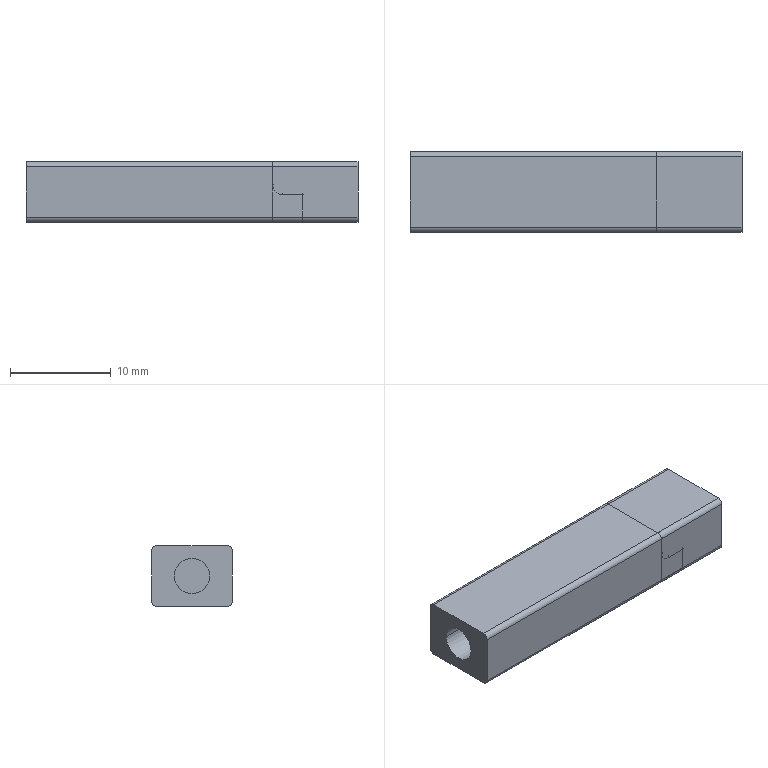NC program | NX | posted with a generic post | part box 33 x 8 x 6 mm
Lines 1895 to 2793 of 11867:
(ZLEVEL_PROFILE_COPY , TOOL : R0.5)
N3746 T13 M6
N3748 G54
N3750 G17 G0 G90 X2.23 Y-1.536 B0. C0. S9500 M3
N3752 G43 Z30. H13
N3754 Z1.5
N3756 G94 G1 X2.302 Y-1.466 Z1.495 F1000.
N3758 X2.547 Y-1.378 Z1.481
N3760 X2.807 Y-1.396 Z1.467
N3762 X3.007 Y-1.494 Z1.456
N3764 X3.168 Y-1.668 Z1.443
N3766 X3.252 Y-1.888 Z1.431
N3768 Y-2.55 Z1.396
N3770 X3.184 Y-2.619 Z1.391
N3772 X2.084 Z1.334
N3774 X2.015 Y-2.55 Z1.328
N3776 Y-1.888 Z1.294
N3778 X2.114 Y-1.647 Z1.28
N3780 X2.302 Y-1.466 Z1.267
N3782 X2.547 Y-1.378 Z1.253
N3784 X2.807 Y-1.396 Z1.239
N3786 X3.007 Y-1.494 Z1.227
N3788 X3.168 Y-1.668 Z1.215
N3790 X3.252 Y-1.888 Z1.203
N3792 Y-2.55 Z1.168
N3794 X3.184 Y-2.619 Z1.163
N3796 X2.084 Z1.105
N3798 X2.015 Y-2.55 Z1.1
N3800 Y-1.888 Z1.066
N3802 X2.114 Y-1.647 Z1.052
N3804 X2.302 Y-1.466 Z1.038
N3806 X2.547 Y-1.378 Z1.025
N3808 X2.807 Y-1.396 Z1.011
N3810 X3.007 Y-1.494 Z0.999
N3812 X3.168 Y-1.668 Z0.987
N3814 X3.252 Y-1.888 Z0.974
N3816 Y-2.55 Z0.94
N3818 X3.184 Y-2.619 Z0.935
N3820 X2.084 Z0.877
N3822 X2.015 Y-2.55 Z0.872
N3824 Y-1.888 Z0.837
N3826 X2.114 Y-1.647 Z0.824
N3828 X2.302 Y-1.466 Z0.81
N3830 X2.547 Y-1.378 Z0.796
N3832 X2.807 Y-1.396 Z0.783
N3834 X3.007 Y-1.494 Z0.771
N3836 X3.168 Y-1.668 Z0.759
N3838 X3.252 Y-1.888 Z0.746
N3840 Y-2.55 Z0.712
N3842 X3.184 Y-2.619 Z0.706
N3844 X2.084 Z0.649
N3846 X2.015 Y-2.55 Z0.644
N3848 Y-1.888 Z0.609
N3850 X2.114 Y-1.647 Z0.595
N3852 X2.302 Y-1.466 Z0.582
N3854 X2.547 Y-1.378 Z0.568
N3856 X2.807 Y-1.396 Z0.554
N3858 X3.007 Y-1.494 Z0.543
N3860 X3.168 Y-1.668 Z0.53
N3862 X3.252 Y-1.888 Z0.518
N3864 Y-2.55 Z0.483
N3866 X3.184 Y-2.619 Z0.478
N3868 X2.084 Z0.421
N3870 X2.015 Y-2.55 Z0.416
N3872 Y-1.888 Z0.381
N3874 X2.114 Y-1.647 Z0.367
N3876 X2.302 Y-1.466 Z0.354
N3878 X2.547 Y-1.378 Z0.34
N3880 X2.807 Y-1.396 Z0.326
N3882 X3.007 Y-1.494 Z0.315
N3884 X3.168 Y-1.668 Z0.302
N3886 X3.252 Y-1.888 Z0.29
N3888 Y-2.55 Z0.255
N3890 X3.184 Y-2.619 Z0.25
N3892 X2.084 Z0.192
N3894 X2.015 Y-2.55 Z0.187
N3896 Y-1.888 Z0.153
N3898 X2.114 Y-1.647 Z0.139
N3900 X2.302 Y-1.466 Z0.125
N3902 X2.547 Y-1.378 Z0.112
N3904 X2.807 Y-1.396 Z0.098
N3906 X3.007 Y-1.494 Z0.086
N3908 X3.168 Y-1.668 Z0.074
N3910 X3.252 Y-1.888 Z0.062
N3912 Y-2.55 Z0.027
N3914 X3.184 Y-2.619 Z0.022
N3916 X2.634 Z-0.007
N3918 X2.134 F2000.
N3920 X2.07 Y-2.611
N3922 X2.023 Y-2.564
N3924 X2.015 Y-2.5
N3926 Y-2.
N3928 G2 X2.634 Y-1.381 R0.619
N3930 X3.252 Y-2. R0.619
N3932 G1 Y-2.5
N3934 X3.245 Y-2.564
N3936 X3.198 Y-2.611
N3938 X3.134 Y-2.619
N3940 X2.634
N3942 X2.571 Y-2.627 Z-0.008
N3944 X2.509 Y-2.636 Z-0.009
N3946 X2.446 Y-2.643 Z-0.01
N3948 X2.384 Y-2.651 Z-0.011
N3950 X2.321 Y-2.658 Z-0.013
N3952 X2.259 Y-2.664 Z-0.014
N3954 X2.196 Y-2.671 Z-0.015
N3956 X2.133 Y-2.677 Z-0.016
N3958 G2 X1.957 Y-2.5 R0.177
N3960 G1 Y-2.
N3962 G2 X2.634 Y-1.323 R0.677
N3964 X3.311 Y-2. R0.677
N3966 G1 Y-2.5
N3968 G2 X3.134 Y-2.677 R0.177
N3970 G1 X2.634
N3972 X2.57 Y-2.683 Z-0.017
N3974 X2.505 Y-2.689 Z-0.018
N3976 X2.441 Y-2.695 Z-0.019
N3978 X2.377 Y-2.7 Z-0.02
N3980 X2.313 Y-2.706 Z-0.021
N3982 X2.248 Y-2.711 Z-0.023
N3984 X2.182 Y-2.716 Z-0.024
N3986 X2.116 Y-2.72 Z-0.025
N3988 X2.074 Y-2.715
N3990 X2.036 Y-2.703 Z-0.026
N3992 X2. Y-2.685
N3994 X1.967 Y-2.66 Z-0.027
N3996 X1.924 Y-2.618
N3998 X1.901 Y-2.561
N4000 X1.903 Y-2.5
N4002 Y-2.
N4004 G2 X2.634 Y-1.269 R0.731
N4006 X3.365 Y-2. R0.731
N4008 G1 Y-2.5
N4010 G2 X3.134 Y-2.731 R0.231
N4012 G1 X2.634
N4014 X2.569 Y-2.736 Z-0.028
N4016 X2.504 Y-2.74 Z-0.029
N4018 X2.439 Y-2.745 Z-0.03
N4020 X2.374 Y-2.749 Z-0.032
N4022 X2.309 Y-2.754 Z-0.033
N4024 X2.244 Y-2.758 Z-0.034
N4026 X2.178 Y-2.762 Z-0.035
N4028 X2.111 Y-2.765 Z-0.036
N4030 X2.072 Y-2.761 Z-0.037
N4032 X2.036 Y-2.752
N4034 X2.001 Y-2.738 Z-0.038
N4036 X1.968 Y-2.718
N4038 X1.937 Y-2.694 Z-0.039
N4040 X1.91 Y-2.665
N4042 X1.888 Y-2.634 Z-0.04
N4044 X1.87 Y-2.599 Z-0.041
N4046 X1.847 Y-2.552
N4048 X1.852 Y-2.5
N4050 Y-2.
N4052 G2 X2.634 Y-1.218 R0.782
N4054 X3.416 Y-2. R0.782
N4056 G1 Y-2.5
N4058 G2 X3.134 Y-2.782 R0.282
N4060 G1 X2.634
N4062 X2.568 Y-2.786 Z-0.042
N4064 X2.502 Y-2.79 Z-0.043
N4066 X2.435 Y-2.794 Z-0.044
N4068 X2.369 Y-2.797 Z-0.045
N4070 X2.303 Y-2.801 Z-0.046
N4072 X2.237 Y-2.805 Z-0.048
N4074 X2.169 Y-2.808 Z-0.049
N4076 X2.101 Y-2.81 Z-0.05
N4078 X2.028 Y-2.797 Z-0.051
N4080 X1.961 Y-2.768 Z-0.052
N4082 X1.9 Y-2.722 Z-0.053
N4084 X1.852 Y-2.664 Z-0.054
N4086 X1.819 Y-2.594 Z-0.056
N4088 X1.802 Y-2.519 Z-0.057
N4090 Y-2.
N4092 G2 X2.634 Y-1.168 R0.832
N4094 X3.466 Y-2. R0.832
N4096 G1 Y-2.5
N4098 G2 X3.134 Y-2.832 R0.332
N4100 G1 X2.634
N4102 X2.568 Y-2.835 Z-0.058
N4104 X2.502 Y-2.839 Z-0.059
N4106 X2.436 Y-2.842 Z-0.06
N4108 X2.37 Y-2.845 Z-0.061
N4110 X2.304 Y-2.848 Z-0.063
N4112 X2.237 Y-2.851 Z-0.064
N4114 X2.17 Y-2.854 Z-0.065
N4116 X2.103 Y-2.856 Z-0.066
N4118 X2.032 Y-2.846 Z-0.067
N4120 X1.965 Y-2.822 Z-0.068
N4122 X1.902 Y-2.784 Z-0.069
N4124 X1.849 Y-2.735 Z-0.071
N4126 X1.805 Y-2.675 Z-0.072
N4128 X1.775 Y-2.608 Z-0.073
N4130 X1.758 Y-2.537 Z-0.074
N4132 X1.753 Y-2.464 Z-0.075
N4134 Y-2.
N4136 G2 X2.634 Y-1.119 R0.881
N4138 X3.515 Y-2. R0.881
N4140 G1 Y-2.5
N4142 G2 X3.134 Y-2.881 R0.381
N4144 G1 X2.634
N4146 X2.568 Y-2.883 Z-0.076
N4148 X2.502 Y-2.886 Z-0.078
N4150 X2.436 Y-2.889 Z-0.079
N4152 X2.37 Y-2.892 Z-0.08
N4154 X2.304 Y-2.894 Z-0.081
N4156 X2.238 Y-2.897 Z-0.082
N4158 X2.171 Y-2.9 Z-0.083
N4160 X2.104 Y-2.901 Z-0.084
N4162 X2.034 Y-2.892 Z-0.086
N4164 X1.967 Y-2.872 Z-0.087
N4166 X1.904 Y-2.839 Z-0.088
N4168 X1.847 Y-2.797 Z-0.089
N4170 X1.798 Y-2.744 Z-0.09
N4172 X1.759 Y-2.684 Z-0.091
N4174 X1.73 Y-2.617 Z-0.093
N4176 X1.714 Y-2.546 Z-0.094
N4178 X1.709 Y-2.478 Z-0.095
N4180 X1.706 Y-2.409 Z-0.096
N4182 Y-2.
N4184 G2 X2.634 Y-1.072 R0.928
N4186 X3.561 Y-2. R0.928
N4188 G1 Y-2.5
N4190 G2 X3.134 Y-2.928 R0.428
N4192 G1 X2.634
N4194 X2.568 Y-2.93 Z-0.097
N4196 X2.502 Y-2.932 Z-0.098
N4198 X2.437 Y-2.935 Z-0.099
N4200 X2.371 Y-2.937 Z-0.101
N4202 X2.305 Y-2.939 Z-0.102
N4204 X2.239 Y-2.942 Z-0.103
N4206 X2.173 Y-2.944 Z-0.104
N4208 X2.106 Y-2.946 Z-0.105
N4210 X2.038 Y-2.938 Z-0.106
N4212 X1.971 Y-2.921 Z-0.107
N4214 X1.907 Y-2.892 Z-0.109
N4216 X1.849 Y-2.855 Z-0.11
N4218 X1.796 Y-2.808 Z-0.111
N4220 X1.751 Y-2.754 Z-0.112
N4222 X1.714 Y-2.693 Z-0.113
N4224 X1.687 Y-2.627 Z-0.114
N4226 X1.671 Y-2.558 Z-0.116
N4228 X1.665 Y-2.487 Z-0.117
N4230 X1.663 Y-2.421 Z-0.118
N4232 X1.661 Y-2.356 Z-0.119
N4234 Y-2.
N4236 G2 X2.634 Y-1.027 R0.973
N4238 X3.607 Y-2. R0.973
N4240 G1 Y-2.5
N4242 G2 X3.134 Y-2.973 R0.473
N4244 G1 X2.634
N4246 X2.568 Y-2.975 Z-0.12
N4248 X2.503 Y-2.977 Z-0.121
N4250 X2.437 Y-2.979 Z-0.122
N4252 X2.371 Y-2.981 Z-0.124
N4254 X2.306 Y-2.984 Z-0.125
N4256 X2.24 Y-2.986 Z-0.126
N4258 X2.174 Y-2.988 Z-0.127
N4260 X2.108 Y-2.989 Z-0.128
N4262 X2.04 Y-2.983 Z-0.129
N4264 X1.973 Y-2.967 Z-0.13
N4266 X1.909 Y-2.942 Z-0.132
N4268 X1.849 Y-2.908 Z-0.133
N4270 X1.794 Y-2.866 Z-0.134
N4272 X1.745 Y-2.817 Z-0.135
N4274 X1.703 Y-2.761 Z-0.136
N4276 X1.669 Y-2.7 Z-0.137
N4278 X1.644 Y-2.634 Z-0.138
N4280 X1.629 Y-2.565 Z-0.14
N4282 X1.622 Y-2.498 Z-0.141
N4284 X1.621 Y-2.429 Z-0.142
N4286 X1.619 Y-2.364 Z-0.143
N4288 X1.617 Y-2.298 Z-0.144
N4290 Y-2.
N4292 G2 X2.634 Y-0.983 R1.017
N4294 X3.651 Y-2. R1.017
N4296 G1 Y-2.5
N4298 G2 X3.134 Y-3.017 R0.517
N4300 G1 X2.634
N4302 X2.569 Y-3.019 Z-0.145
N4304 X2.504 Y-3.021 Z-0.146
N4306 X2.438 Y-3.023 Z-0.148
N4308 X2.373 Y-3.025 Z-0.149
N4310 X2.308 Y-3.027 Z-0.15
N4312 X2.243 Y-3.028 Z-0.151
N4314 X2.177 Y-3.03 Z-0.152
N4316 X2.112 Y-3.032 Z-0.153
N4318 X2.045 Y-3.026 Z-0.154
N4320 X1.979 Y-3.013 Z-0.156
N4322 X1.915 Y-2.991 Z-0.157
N4324 X1.854 Y-2.961 Z-0.158
N4326 X1.797 Y-2.923 Z-0.159
N4328 X1.746 Y-2.879 Z-0.16
N4330 X1.699 Y-2.828 Z-0.161
N4332 X1.66 Y-2.772 Z-0.162
N4334 X1.628 Y-2.711 Z-0.164
N4336 X1.604 Y-2.646 Z-0.165
N4338 X1.588 Y-2.579 Z-0.166
N4340 X1.581 Y-2.51 Z-0.167
N4342 X1.579 Y-2.444 Z-0.168
N4344 X1.577 Y-2.379 Z-0.169
N4346 X1.576 Y-2.313 Z-0.17
N4348 X1.574 Y-2.248 Z-0.171
N4350 Y-2.
N4352 G2 X2.634 Y-0.94 R1.06
N4354 X3.694 Y-2. R1.06
N4356 G1 Y-2.5
N4358 G2 X3.134 Y-3.06 R0.56
N4360 G1 X2.634
N4362 X2.564 Y-3.062 Z-0.173
N4364 X2.494 Y-3.064 Z-0.174
N4366 X2.424 Y-3.065 Z-0.175
N4368 X2.353 Y-3.067 Z-0.176
N4370 X2.283 Y-3.069 Z-0.178
N4372 X2.213 Y-3.071 Z-0.179
N4374 X2.142 Y-3.072 Z-0.18
N4376 X2.072 Y-3.071 Z-0.181
N4378 X2. Y-3.06 Z-0.183
N4380 X1.931 Y-3.041 Z-0.184
N4382 X1.864 Y-3.013 Z-0.185
N4384 X1.801 Y-2.976 Z-0.186
N4386 X1.743 Y-2.932 Z-0.187
N4388 X1.691 Y-2.881 Z-0.189
N4390 X1.645 Y-2.824 Z-0.19
N4392 X1.607 Y-2.761 Z-0.191
N4394 X1.577 Y-2.694 Z-0.192
N4396 X1.556 Y-2.623 Z-0.194
N4398 X1.543 Y-2.551 Z-0.195
N4400 X1.539 Y-2.477 Z-0.196
N4402 X1.538 Y-2.407 Z-0.197
N4404 X1.536 Y-2.337 Z-0.198
N4406 X1.534 Y-2.267 Z-0.2
N4408 X1.533 Y-2.197 Z-0.201
N4410 Y-2.
N4412 G2 X2.634 Y-0.899 R1.101
N4414 X3.735 Y-2. R1.101
N4416 G1 Y-2.5
N4418 G2 X3.134 Y-3.101 R0.601
N4420 G1 X2.634
N4422 X2.565 Y-3.103 Z-0.202
N4424 X2.496 Y-3.104 Z-0.203
N4426 X2.427 Y-3.106 Z-0.204
N4428 X2.357 Y-3.108 Z-0.206
N4430 X2.288 Y-3.109 Z-0.207
N4432 X2.219 Y-3.111 Z-0.208
N4434 X2.149 Y-3.112 Z-0.209
N4436 X2.08 Y-3.111 Z-0.211
N4438 X2.01 Y-3.103 Z-0.212
N4440 X1.941 Y-3.086 Z-0.213
N4442 X1.874 Y-3.061 Z-0.214
N4444 X1.811 Y-3.029 Z-0.215
N4446 X1.751 Y-2.99 Z-0.217
N4448 X1.697 Y-2.944 Z-0.218
N4450 X1.647 Y-2.891 Z-0.219
N4452 X1.604 Y-2.834 Z-0.22
N4454 X1.568 Y-2.771 Z-0.221
N4456 X1.539 Y-2.705 Z-0.223
N4458 X1.518 Y-2.636 Z-0.224
N4460 X1.505 Y-2.565 Z-0.225
N4462 X1.501 Y-2.494 Z-0.226
N4464 X1.499 Y-2.423 Z-0.227
N4466 X1.498 Y-2.354 Z-0.229
N4468 X1.496 Y-2.285 Z-0.23
N4470 X1.495 Y-2.216 Z-0.231
N4472 X1.493 Y-2.147 Z-0.232
N4474 Y-2.
N4476 G2 X2.634 Y-0.859 R1.141
N4478 X3.775 Y-2. R1.141
N4480 G1 Y-2.5
N4482 G2 X3.134 Y-3.141 R0.641
N4484 G1 X2.634
N4486 X2.566 Y-3.142 Z-0.233
N4488 X2.498 Y-3.144 Z-0.235
N4490 X2.43 Y-3.145 Z-0.236
N4492 X2.362 Y-3.146 Z-0.237
N4494 X2.294 Y-3.148 Z-0.238
N4496 X2.225 Y-3.149 Z-0.239
N4498 X2.157 Y-3.151 Z-0.241
N4500 X2.089 Y-3.15 Z-0.242
N4502 X2.019 Y-3.143 Z-0.243
N4504 X1.952 Y-3.129 Z-0.244
N4506 X1.885 Y-3.107 Z-0.245
N4508 X1.822 Y-3.079 Z-0.247
N4510 X1.761 Y-3.043 Z-0.248
N4512 X1.705 Y-3.002 Z-0.249
N4514 X1.653 Y-2.954 Z-0.25
N4516 X1.607 Y-2.902 Z-0.251
N4518 X1.566 Y-2.844 Z-0.252
N4520 X1.531 Y-2.783 Z-0.254
N4522 X1.504 Y-2.717 Z-0.255
N4524 X1.483 Y-2.65 Z-0.256
N4526 X1.469 Y-2.58 Z-0.257
N4528 X1.463 Y-2.509 Z-0.258
N4530 X1.462 Y-2.441 Z-0.26
N4532 X1.461 Y-2.372 Z-0.261
N4534 X1.459 Y-2.304 Z-0.262
N4536 X1.458 Y-2.236 Z-0.263
N4538 X1.457 Y-2.168 Z-0.264
N4540 X1.455 Y-2.1 Z-0.266
N4542 Y-2.
N4544 G2 X2.634 Y-0.821 R1.179
N4546 X3.813 Y-2. R1.179
N4548 G1 Y-2.5
N4550 G2 X3.134 Y-3.179 R0.679
N4552 G1 X2.634
N4554 X2.567 Y-3.18 Z-0.267
N4556 X2.5 Y-3.181 Z-0.268
N4558 X2.433 Y-3.182 Z-0.269
N4560 X2.366 Y-3.184 Z-0.27
N4562 X2.299 Y-3.185 Z-0.271
N4564 X2.232 Y-3.186 Z-0.273
N4566 X2.165 Y-3.187 Z-0.274
N4568 X2.097 Y-3.188 Z-0.275
N4570 X2.03 Y-3.182 Z-0.276
N4572 X1.963 Y-3.169 Z-0.277
N4574 X1.897 Y-3.15 Z-0.278
N4576 X1.834 Y-3.125 Z-0.28
N4578 X1.773 Y-3.093 Z-0.281
N4580 X1.715 Y-3.056 Z-0.282
N4582 X1.662 Y-3.013 Z-0.283
N4584 X1.613 Y-2.965 Z-0.284
N4586 X1.568 Y-2.912 Z-0.285
N4588 X1.53 Y-2.854 Z-0.287
N4590 X1.496 Y-2.794 Z-0.288
N4592 X1.469 Y-2.73 Z-0.289
N4594 X1.449 Y-2.663 Z-0.29
N4596 X1.435 Y-2.595 Z-0.291
N4598 X1.428 Y-2.527 Z-0.292
N4600 X1.426 Y-2.458 Z-0.294
N4602 X1.425 Y-2.391 Z-0.295
N4604 X1.424 Y-2.324 Z-0.296
N4606 X1.423 Y-2.257 Z-0.297
N4608 X1.422 Y-2.19 Z-0.298
N4610 X1.42 Y-2.123 Z-0.299
N4612 X1.419 Y-2.056 Z-0.301
N4614 Y-2.
N4616 G2 X2.634 Y-0.785 R1.215
N4618 X3.849 Y-2. R1.215
N4620 G1 Y-2.5
N4622 G2 X3.134 Y-3.215 R0.715
N4624 G1 X2.634
N4626 X2.564 Y-3.216 Z-0.302
N4628 X2.493 Y-3.217 Z-0.303
N4630 X2.423 Y-3.218 Z-0.304
N4632 X2.353 Y-3.22 Z-0.306
N4634 X2.282 Y-3.221 Z-0.307
N4636 X2.212 Y-3.222 Z-0.308
N4638 X2.141 Y-3.223 Z-0.309
N4640 X2.07 Y-3.221 Z-0.31
N4642 X2. Y-3.213 Z-0.312
N4644 X1.93 Y-3.197 Z-0.313
N4646 X1.862 Y-3.175 Z-0.314
N4648 X1.796 Y-3.146 Z-0.315
N4650 X1.734 Y-3.111 Z-0.317
N4652 X1.675 Y-3.069 Z-0.318
N4654 X1.621 Y-3.022 Z-0.319
N4656 X1.571 Y-2.97 Z-0.32
N4658 X1.527 Y-2.913 Z-0.321
N4660 X1.488 Y-2.852 Z-0.323
N4662 X1.455 Y-2.787 Z-0.324
N4664 X1.429 Y-2.72 Z-0.325
N4666 X1.41 Y-2.649 Z-0.326
N4668 X1.398 Y-2.578 Z-0.328
N4670 X1.393 Y-2.506 Z-0.329
N4672 X1.392 Y-2.434 Z-0.33
N4674 X1.39 Y-2.364 Z-0.331
N4676 X1.389 Y-2.294 Z-0.333
N4678 X1.388 Y-2.223 Z-0.334
N4680 X1.387 Y-2.153 Z-0.335
N4682 X1.386 Y-2.083 Z-0.336
N4684 X1.385 Y-2.012 Z-0.337
N4686 Y-2.
N4688 G2 X2.634 Y-0.751 R1.249
N4690 X3.883 Y-2. R1.249
N4692 G1 Y-2.5
N4694 G2 X3.134 Y-3.249 R0.749
N4696 G1 X2.634
N4698 X2.565 Y-3.25 Z-0.339
N4700 X2.496 Y-3.251 Z-0.34
N4702 X2.427 Y-3.252 Z-0.341
N4704 X2.358 Y-3.253 Z-0.342
N4706 X2.29 Y-3.254 Z-0.343
N4708 X2.221 Y-3.255 Z-0.345
N4710 X2.151 Y-3.256 Z-0.346
N4712 X2.082 Z-0.347
N4714 X2.013 Y-3.249 Z-0.348
N4716 X1.944 Y-3.235 Z-0.349
N4718 X1.877 Y-3.216 Z-0.351
N4720 X1.812 Y-3.19 Z-0.352
N4722 X1.75 Y-3.159 Z-0.353
N4724 X1.69 Y-3.121 Z-0.354
N4726 X1.634 Y-3.079 Z-0.355
N4728 X1.583 Y-3.031 Z-0.357
N4730 X1.535 Y-2.979 Z-0.358
N4732 X1.493 Y-2.922 Z-0.359
N4734 X1.456 Y-2.862 Z-0.36
N4736 X1.425 Y-2.799 Z-0.361
N4738 X1.399 Y-2.733 Z-0.363
N4740 X1.38 Y-2.665 Z-0.364
N4742 X1.367 Y-2.595 Z-0.365
N4744 X1.361 Y-2.524 Z-0.366
N4746 X1.359 Y-2.455 Z-0.367
N4748 X1.358 Y-2.385 Z-0.369
N4750 X1.357 Y-2.317 Z-0.37
N4752 X1.356 Y-2.248 Z-0.371
N4754 Y-2.179 Z-0.372
N4756 X1.355 Y-2.11 Z-0.374
N4758 X1.354 Y-2.041 Z-0.375
N4760 X1.353 Y-1.971 Z-0.376
N4762 G2 X3.915 Y-2. R1.281
N4764 G1 Y-2.5
N4766 G2 X3.134 Y-3.281 R0.781
N4768 G1 X2.634
N4770 X2.567 Y-3.282 Z-0.377
N4772 X2.499 Y-3.283 Z-0.378
N4774 X2.432 Y-3.284 Z-0.379
N4776 X2.364 Y-3.285 Z-0.381
N4778 X2.297 Y-3.286 Z-0.382
N4780 X2.229 Y-3.287 Z-0.383
N4782 X2.162 Y-3.288 Z-0.384
N4784 X2.094 Z-0.385
N4786 X2.026 Y-3.282 Z-0.387
N4788 X1.959 Y-3.271 Z-0.388
N4790 X1.893 Y-3.254 Z-0.389
N4792 X1.828 Y-3.231 Z-0.39
N4794 X1.766 Y-3.203 Z-0.391
N4796 X1.706 Y-3.169 Z-0.392
N4798 X1.65 Y-3.131 Z-0.394
N4800 X1.597 Y-3.087 Z-0.395
N4802 X1.547 Y-3.039 Z-0.396
N4804 X1.502 Y-2.987 Z-0.397
N4806 X1.462 Y-2.932 Z-0.398
N4808 X1.426 Y-2.872 Z-0.399
N4810 X1.396 Y-2.81 Z-0.401
N4812 X1.371 Y-2.746 Z-0.402
N4814 X1.352 Y-2.679 Z-0.403
N4816 X1.339 Y-2.612 Z-0.404
N4818 X1.331 Y-2.543 Z-0.405
N4820 X1.329 Y-2.474 Z-0.407
N4822 X1.328 Y-2.407 Z-0.408
N4824 X1.327 Y-2.339 Z-0.409
N4826 Y-2.272 Z-0.41
N4828 X1.326 Y-2.204 Z-0.411
N4830 X1.325 Y-2.137 Z-0.412
N4832 X1.324 Y-2.069 Z-0.414
N4834 X1.323 Y-2.001 Z-0.415
N4836 X1.324 Y-1.933 Z-0.416
N4838 G2 X3.946 Y-2. R1.312
N4840 G1 Y-2.5
N4842 G2 X3.134 Y-3.312 R0.812
N4844 G1 X2.634
N4846 X2.564 Y-3.313 Z-0.417
N4848 X2.494 Z-0.418
N4850 X2.424 Y-3.314 Z-0.42
N4852 X2.354 Y-3.315 Z-0.421
N4854 X2.285 Y-3.316 Z-0.422
N4856 X2.215 Y-3.317 Z-0.423
N4858 X2.145 Y-3.318 Z-0.424
N4860 X2.075 Y-3.316 Z-0.426
N4862 X2.004 Y-3.309 Z-0.427
N4864 X1.935 Y-3.296 Z-0.428
N4866 X1.867 Y-3.277 Z-0.429
N4868 X1.801 Y-3.252 Z-0.431
N4870 X1.737 Y-3.221 Z-0.432
N4872 X1.676 Y-3.185 Z-0.433
N4874 X1.619 Y-3.144 Z-0.434
N4876 X1.565 Y-3.098 Z-0.435
N4878 X1.515 Y-3.047 Z-0.437
N4880 X1.469 Y-2.992 Z-0.438
N4882 X1.429 Y-2.934 Z-0.439
N4884 X1.393 Y-2.872 Z-0.44
N4886 X1.363 Y-2.807 Z-0.442
N4888 X1.339 Y-2.74 Z-0.443
N4890 X1.321 Y-2.671 Z-0.444
N4892 X1.308 Y-2.6 Z-0.445
N4894 X1.302 Y-2.53 Z-0.446
N4896 X1.3 Y-2.458 Z-0.448
N4898 Y-2.389 Z-0.449
N4900 X1.299 Y-2.319 Z-0.45
N4902 X1.298 Y-2.249 Z-0.451
N4904 X1.297 Y-2.179 Z-0.453
N4906 X1.296 Y-2.109 Z-0.454
N4908 Y-2.039 Z-0.455
N4910 X1.295 Y-1.968 Z-0.456
N4912 X1.298 Y-1.897 Z-0.457
N4914 G2 X3.974 Y-2. R1.34
N4916 G1 Y-2.5
N4918 G2 X3.134 Y-3.34 R0.84
N4920 G1 X2.634
N4922 X2.566 Y-3.341 Z-0.459
N4924 X2.498 Y-3.342 Z-0.46
N4926 X2.43 Z-0.461
N4928 X2.361 Y-3.343 Z-0.462
N4930 X2.293 Y-3.344 Z-0.463
N4932 X2.225 Y-3.345 Z-0.465
N4934 X2.157 Z-0.466
N4936 X2.089 Z-0.467
N4938 X2.02 Y-3.339 Z-0.468
N4940 X1.952 Y-3.328 Z-0.469
N4942 X1.886 Y-3.311 Z-0.47
N4944 X1.821 Y-3.289 Z-0.472
N4946 X1.757 Y-3.262 Z-0.473
N4948 X1.696 Y-3.229 Z-0.474
N4950 X1.638 Y-3.192 Z-0.475
N4952 X1.583 Y-3.15 Z-0.476
N4954 X1.532 Y-3.104 Z-0.478
N4956 X1.485 Y-3.054 Z-0.479
N4958 X1.441 Y-3. Z-0.48
N4960 X1.402 Y-2.942 Z-0.481
N4962 X1.368 Y-2.882 Z-0.482
N4964 X1.339 Y-2.819 Z-0.484
N4966 X1.315 Y-2.754 Z-0.485
N4968 X1.297 Y-2.687 Z-0.486
N4970 X1.284 Y-2.618 Z-0.487
N4972 X1.276 Y-2.549 Z-0.488
N4974 X1.274 Y-2.48 Z-0.49
N4976 X1.273 Y-2.412 Z-0.491
N4978 Y-2.344 Z-0.492
N4980 X1.272 Y-2.276 Z-0.493
N4982 X1.271 Y-2.207 Z-0.494
N4984 Y-2.139 Z-0.495
N4986 X1.27 Y-2.071 Z-0.497
N4988 X1.269 Y-2.003 Z-0.498
N4990 X1.27 Y-1.934 Z-0.499
N4992 X1.275 Y-1.864 Z-0.5
N4994 G2 X4. Y-2. R1.366
N4996 G1 Y-2.5
N4998 G2 X3.134 Y-3.366 R0.866
N5000 G1 X2.634
N5002 X2.564 Y-3.367 Z-0.501
N5004 X2.494 Y-3.368 Z-0.503
N5006 X2.424 Z-0.504
N5008 X2.354 Y-3.369 Z-0.505
N5010 X2.283 Y-3.37 Z-0.506
N5012 X2.213 Z-0.508
N5014 X2.143 Y-3.371 Z-0.509
N5016 X2.073 Y-3.37 Z-0.51
N5018 X2.003 Y-3.362 Z-0.511
N5020 X1.933 Y-3.35 Z-0.512
N5022 X1.865 Y-3.331 Z-0.514
N5024 X1.798 Y-3.307 Z-0.515
N5026 X1.734 Y-3.278 Z-0.516
N5028 X1.672 Y-3.244 Z-0.517
N5030 X1.613 Y-3.205 Z-0.519
N5032 X1.557 Y-3.161 Z-0.52
N5034 X1.505 Y-3.112 Z-0.521
N5036 X1.457 Y-3.06 Z-0.522
N5038 X1.413 Y-3.004 Z-0.523
N5040 X1.375 Y-2.944 Z-0.525
N5042 X1.34 Y-2.882 Z-0.526
N5044 X1.312 Y-2.816 Z-0.527
N5046 X1.288 Y-2.749 Z-0.528
N5048 X1.27 Y-2.68 Z-0.53
N5050 X1.258 Y-2.61 Z-0.531
N5052 X1.251 Y-2.538 Z-0.532
N5054 X1.25 Y-2.468 Z-0.533
N5056 X1.249 Y-2.398 Z-0.534
N5058 X1.248 Y-2.327 Z-0.536
N5060 Y-2.257 Z-0.537
N5062 X1.247 Y-2.187 Z-0.538
N5064 X1.246 Y-2.117 Z-0.539
N5066 Y-2.047 Z-0.541
N5068 X1.245 Y-1.976 Z-0.542
N5070 X1.248 Y-1.905 Z-0.543
N5072 X1.254 Y-1.834 Z-0.544
N5074 G2 X4.024 Y-2. R1.39
N5076 G1 Y-2.5
N5078 G2 X3.134 Y-3.39 R0.89
N5080 G1 X2.634
N5082 X2.566 Y-3.391 Z-0.545
N5084 X2.498 Z-0.547
N5086 X2.43 Y-3.392 Z-0.548
N5088 X2.362 Y-3.393 Z-0.549
N5090 X2.293 Z-0.55
N5092 X2.225 Y-3.394 Z-0.551
N5094 X2.157 Z-0.553
N5096 X2.089 Z-0.554
N5098 X2.021 Y-3.388 Z-0.555
N5100 X1.953 Y-3.378 Z-0.556
N5102 X1.886 Y-3.362 Z-0.557
N5104 X1.821 Y-3.341 Z-0.559
N5106 X1.757 Y-3.315 Z-0.56
N5108 X1.696 Y-3.284 Z-0.561
N5110 X1.637 Y-3.249 Z-0.562
N5112 X1.581 Y-3.209 Z-0.563
N5114 X1.528 Y-3.165 Z-0.564
N5116 X1.478 Y-3.118 Z-0.566
N5118 X1.432 Y-3.066 Z-0.567
N5120 X1.391 Y-3.011 Z-0.568
N5122 X1.353 Y-2.953 Z-0.569
N5124 X1.321 Y-2.892 Z-0.57
N5126 X1.292 Y-2.829 Z-0.572
N5128 X1.269 Y-2.764 Z-0.573
N5130 X1.251 Y-2.697 Z-0.574
N5132 X1.238 Y-2.629 Z-0.575
N5134 X1.23 Y-2.56 Z-0.576
N5136 X1.228 Y-2.491 Z-0.578
N5138 X1.227 Y-2.423 Z-0.579
N5140 X1.226 Y-2.355 Z-0.58
N5142 Y-2.287 Z-0.581
N5144 X1.225 Y-2.219 Z-0.582
N5146 Y-2.151 Z-0.583
N5148 X1.224 Y-2.083 Z-0.585
N5150 Y-2.014 Z-0.586
N5152 Y-1.946 Z-0.587
N5154 X1.228 Y-1.877 Z-0.588
N5156 X1.235 Y-1.808 Z-0.589
N5158 G2 X4.046 Y-2. R1.412
N5160 G1 Y-2.5
N5162 G2 X3.134 Y-3.412 R0.912
N5164 G1 X2.634
N5166 X2.564 Z-0.591
N5168 X2.495 Y-3.413 Z-0.592
N5170 X2.425 Z-0.593
N5172 X2.355 Y-3.414 Z-0.594
N5174 X2.286 Y-3.415 Z-0.596
N5176 X2.216 Z-0.597
N5178 X2.146 Y-3.416 Z-0.598
N5180 X2.077 Y-3.414 Z-0.599
N5182 X2.007 Y-3.408 Z-0.6
N5184 X1.938 Y-3.396 Z-0.602
N5186 X1.87 Y-3.379 Z-0.603
N5188 X1.803 Y-3.357 Z-0.604
N5190 X1.739 Y-3.329 Z-0.605
N5192 X1.676 Y-3.297 Z-0.606
N5194 X1.617 Y-3.261 Z-0.608
N5196 X1.56 Y-3.219 Z-0.609
N5198 X1.506 Y-3.174 Z-0.61
N5200 X1.456 Y-3.124 Z-0.611
N5202 X1.41 Y-3.071 Z-0.613
N5204 X1.368 Y-3.014 Z-0.614
N5206 X1.331 Y-2.955 Z-0.615
N5208 X1.298 Y-2.892 Z-0.616
N5210 X1.27 Y-2.828 Z-0.617
N5212 X1.247 Y-2.761 Z-0.619
N5214 X1.229 Y-2.692 Z-0.62
N5216 X1.217 Y-2.623 Z-0.621
N5218 X1.21 Y-2.553 Z-0.622
N5220 X1.208 Y-2.482 Z-0.623
N5222 X1.207 Y-2.413 Z-0.625
N5224 Y-2.343 Z-0.626
N5226 X1.206 Y-2.273 Z-0.627
N5228 Y-2.204 Z-0.628
N5230 X1.205 Y-2.134 Z-0.63
N5232 Y-2.064 Z-0.631
N5234 X1.204 Y-1.994 Z-0.632
N5236 X1.206 Y-1.924 Z-0.633
N5238 X1.211 Y-1.854 Z-0.634
N5240 X1.219 Y-1.784 Z-0.636
N5242 G2 X4.065 Y-2. R1.431
N5244 G1 Y-2.5
N5246 G2 X3.134 Y-3.431 R0.931
N5248 G1 X2.634
N5250 X2.567 Y-3.432 Z-0.637
N5252 X2.499 Z-0.638
N5254 X2.432 Y-3.433 Z-0.639
N5256 X2.364 Z-0.64
N5258 X2.297 Y-3.434 Z-0.642
N5260 X2.229 Z-0.643
N5262 X2.162 Z-0.644
N5264 X2.094 Z-0.645
N5266 X2.027 Y-3.429 Z-0.646
N5268 X1.96 Y-3.419 Z-0.647
N5270 X1.894 Y-3.405 Z-0.649
N5272 X1.829 Y-3.385 Z-0.65
N5274 X1.765 Y-3.361 Z-0.651
N5276 X1.704 Y-3.333 Z-0.652
N5278 X1.644 Y-3.3 Z-0.653
N5280 X1.587 Y-3.263 Z-0.654
N5282 X1.533 Y-3.222 Z-0.656
N5284 X1.482 Y-3.176 Z-0.657
N5286 X1.435 Y-3.128 Z-0.658
N5288 X1.391 Y-3.076 Z-0.659
N5290 X1.351 Y-3.021 Z-0.66
N5292 X1.315 Y-2.963 Z-0.662
N5294 X1.283 Y-2.903 Z-0.663
N5296 X1.256 Y-2.84 Z-0.664
N5298 X1.233 Y-2.776 Z-0.665
N5300 X1.215 Y-2.71 Z-0.666
N5302 X1.202 Y-2.643 Z-0.667
N5304 X1.193 Y-2.575 Z-0.669
N5306 X1.19 Y-2.507 Z-0.67
N5308 Y-2.44 Z-0.671
N5310 X1.189 Y-2.372 Z-0.672
N5312 Y-2.305 Z-0.673
N5314 X1.188 Y-2.237 Z-0.674
N5316 Y-2.17 Z-0.676
N5318 Y-2.102 Z-0.677
N5320 X1.187 Y-2.035 Z-0.678
N5322 Y-1.967 Z-0.679
N5324 X1.19 Y-1.899 Z-0.68
N5326 X1.196 Y-1.831 Z-0.682
N5328 X1.205 Y-1.763 Z-0.683
N5330 G2 X4.082 Y-2. R1.448
N5332 G1 Y-2.5
N5334 G2 X3.134 Y-3.448 R0.948
N5336 G1 X2.634
N5338 X2.565 Y-3.449 Z-0.684
N5340 X2.497 Z-0.685
N5342 X2.428 Y-3.45 Z-0.686
N5344 X2.36 Z-0.688
N5346 X2.291 Z-0.689
N5348 X2.223 Y-3.451 Z-0.69
N5350 X2.154 Z-0.691
N5352 X2.085 Y-3.45 Z-0.692
N5354 X2.017 Y-3.445 Z-0.693
N5356 X1.949 Y-3.434 Z-0.695
N5358 X1.882 Y-3.419 Z-0.696
N5360 X1.816 Y-3.398 Z-0.697
N5362 X1.752 Y-3.373 Z-0.698
N5364 X1.689 Y-3.344 Z-0.699
N5366 X1.629 Y-3.31 Z-0.701
N5368 X1.572 Y-3.272 Z-0.702
N5370 X1.518 Y-3.229 Z-0.703
N5372 X1.466 Y-3.183 Z-0.704
N5374 X1.418 Y-3.133 Z-0.705
N5376 X1.374 Y-3.08 Z-0.707
N5378 X1.334 Y-3.024 Z-0.708
N5380 X1.298 Y-2.965 Z-0.709
N5382 X1.266 Y-2.904 Z-0.71
N5384 X1.239 Y-2.84 Z-0.711
N5386 X1.216 Y-2.774 Z-0.713
N5388 X1.199 Y-2.708 Z-0.714
N5390 X1.186 Y-2.64 Z-0.715
N5392 X1.178 Y-2.571 Z-0.716
N5394 X1.175 Y-2.502 Z-0.717
N5396 X1.174 Y-2.433 Z-0.719
N5398 Y-2.364 Z-0.72
N5400 Y-2.296 Z-0.721
N5402 X1.173 Y-2.227 Z-0.722
N5404 Y-2.159 Z-0.723
N5406 Y-2.09 Z-0.725
N5408 X1.172 Y-2.022 Z-0.726
N5410 X1.173 Y-1.952 Z-0.727
N5412 X1.176 Y-1.883 Z-0.728
N5414 X1.183 Y-1.814 Z-0.729
N5416 X1.193 Y-1.746 Z-0.731
N5418 G2 X4.097 Y-2. R1.463
N5420 G1 Y-2.5
N5422 G2 X3.134 Y-3.463 R0.963
N5424 G1 X2.634
N5426 X2.564 Z-0.732
N5428 X2.495 Y-3.464 Z-0.733
N5430 X2.425 Z-0.734
N5432 X2.356 Z-0.735
N5434 X2.286 Y-3.465 Z-0.737
N5436 X2.217 Z-0.738
N5438 X2.147 Z-0.739
N5440 X2.078 Y-3.464 Z-0.74
N5442 X2.008 Y-3.458 Z-0.742
N5444 X1.94 Y-3.447 Z-0.743
N5446 X1.872 Y-3.43 Z-0.744
N5448 X1.805 Y-3.409 Z-0.745
N5450 X1.74 Y-3.384 Z-0.746
N5452 X1.678 Y-3.353 Z-0.748
N5454 X1.617 Y-3.318 Z-0.749
N5456 X1.559 Y-3.279 Z-0.75
N5458 X1.504 Y-3.236 Z-0.751
N5460 X1.453 Y-3.189 Z-0.752
N5462 X1.404 Y-3.138 Z-0.754
N5464 X1.36 Y-3.084 Z-0.755
N5466 X1.32 Y-3.027 Z-0.756
N5468 X1.284 Y-2.967 Z-0.757
N5470 X1.252 Y-2.904 Z-0.758
N5472 X1.225 Y-2.84 Z-0.76
N5474 X1.202 Y-2.774 Z-0.761
N5476 X1.185 Y-2.706 Z-0.762
N5478 X1.172 Y-2.637 Z-0.763
N5480 X1.164 Y-2.567 Z-0.765
N5482 X1.162 Y-2.497 Z-0.766
N5484 Y-2.428 Z-0.767
N5486 X1.161 Y-2.358 Z-0.768
N5488 Y-2.289 Z-0.769
N5490 Y-2.219 Z-0.771
N5492 X1.16 Y-2.15 Z-0.772
N5494 Y-2.08 Z-0.773
N5496 Y-2.01 Z-0.774
N5498 X1.161 Y-1.94 Z-0.775
N5500 X1.165 Y-1.871 Z-0.777
N5502 X1.172 Y-1.801 Z-0.778
N5504 X1.183 Y-1.732 Z-0.779
N5506 G2 X4.109 Y-2. R1.475
N5508 G1 Y-2.5
N5510 G2 X3.134 Y-3.475 R0.975
N5512 G1 X2.634
N5514 X2.564 Y-3.476 Z-0.78
N5516 X2.493 Z-0.782
N5518 X2.423 Z-0.783
N5520 X2.353 Z-0.784
N5522 X2.283 Y-3.477 Z-0.785
N5524 X2.212 Z-0.786
N5526 X2.142 Z-0.788
N5528 X2.072 Y-3.475 Z-0.789
N5530 X2.002 Y-3.469 Z-0.79
N5532 X1.932 Y-3.457 Z-0.791
N5534 X1.864 Y-3.44 Z-0.793
N5536 X1.797 Y-3.419 Z-0.794